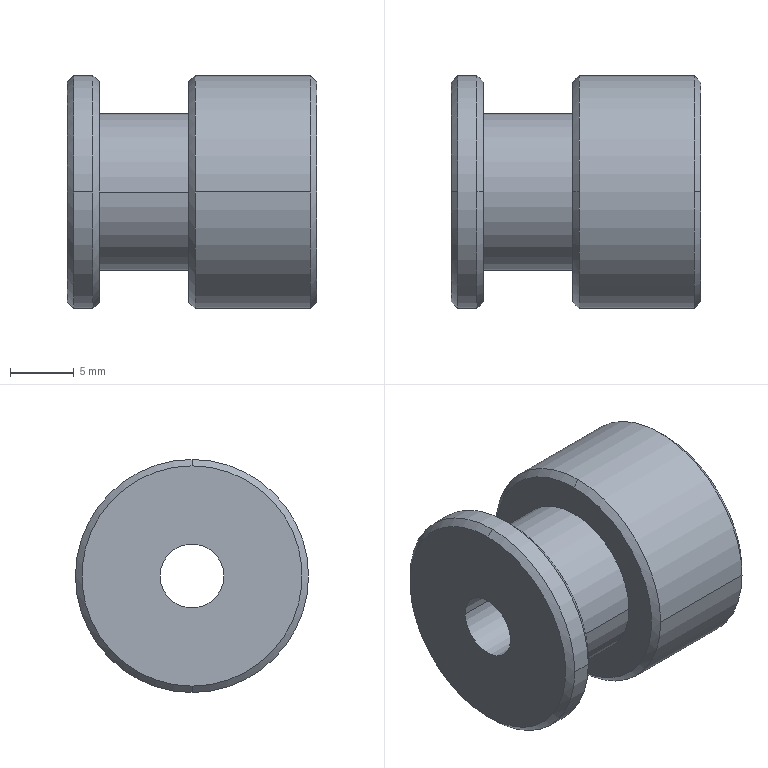Part | SolidWorks | features BaseBody 1 | 1 solid | 20 faces | box 19.5 x 18.22 x 18.22 mm | volume 3669 mm3 | cylinder 8 | cone 8 | plane 4 | commonest cylinder face diameters 18.22 x4 5 x2 12.22 x2
STEP:
#1=CARTESIAN_POINT('',(-10.344,-4.715,9.11));
#2=VERTEX_POINT('',#1);
#3=CARTESIAN_POINT('',(-10.344,-13.825,0.));
#4=VERTEX_POINT('',#3);
#5=CARTESIAN_POINT('',(-10.344,-4.715,0.));
#6=DIRECTION('',(1.,0.,0.));
#7=DIRECTION('',(0.,1.,0.));
#8=AXIS2_PLACEMENT_3D('',#5,#6,#7);
#9=CIRCLE('',#8,9.11);
#10=EDGE_CURVE('',#2,#4,#9,.T.);
#11=ORIENTED_EDGE('',*,*,#10,.T.);
#12=CARTESIAN_POINT('',(-1.344,-13.825,0.));
#13=VERTEX_POINT('',#12);
#14=CARTESIAN_POINT('',(-5.844,-13.825,0.));
#15=DIRECTION('',(1.,0.,0.));
#16=VECTOR('',#15,1000.);
#17=LINE('',#14,#16);
#18=EDGE_CURVE('',#4,#13,#17,.T.);
#19=ORIENTED_EDGE('',*,*,#18,.T.);
#20=CARTESIAN_POINT('',(-1.344,-4.715,9.11));
#21=VERTEX_POINT('',#20);
#22=CARTESIAN_POINT('',(-1.344,-4.715,0.));
#23=DIRECTION('',(-1.,0.,0.));
#24=DIRECTION('',(0.,1.,0.));
#25=AXIS2_PLACEMENT_3D('',#22,#23,#24);
#26=CIRCLE('',#25,9.11);
#27=EDGE_CURVE('',#13,#21,#26,.T.);
#28=ORIENTED_EDGE('',*,*,#27,.T.);
#29=CARTESIAN_POINT('',(-1.344,4.395,0.));
#30=VERTEX_POINT('',#29);
#31=CARTESIAN_POINT('',(-1.344,-4.715,0.));
#32=DIRECTION('',(-1.,0.,0.));
#33=DIRECTION('',(0.,1.,0.));
#34=AXIS2_PLACEMENT_3D('',#31,#32,#33);
#35=CIRCLE('',#34,9.11);
#36=EDGE_CURVE('',#21,#30,#35,.T.);
#37=ORIENTED_EDGE('',*,*,#36,.T.);
#38=CARTESIAN_POINT('',(-10.344,4.395,0.));
#39=VERTEX_POINT('',#38);
#40=CARTESIAN_POINT('',(-5.844,4.395,0.));
#41=DIRECTION('',(1.,0.,0.));
#42=VECTOR('',#41,1000.);
#43=LINE('',#40,#42);
#44=EDGE_CURVE('',#39,#30,#43,.T.);
#45=ORIENTED_EDGE('',*,*,#44,.F.);
#46=CARTESIAN_POINT('',(-10.344,-4.715,0.));
#47=DIRECTION('',(1.,0.,0.));
#48=DIRECTION('',(0.,1.,0.));
#49=AXIS2_PLACEMENT_3D('',#46,#47,#48);
#50=CIRCLE('',#49,9.11);
#51=EDGE_CURVE('',#39,#2,#50,.T.);
#52=ORIENTED_EDGE('',*,*,#51,.T.);
#53=EDGE_LOOP('',(#11,#19,#28,#37,#45,#52));
#54=FACE_OUTER_BOUND('',#53,.T.);
#55=CARTESIAN_POINT('',(-5.844,-4.715,0.));
#56=DIRECTION('',(1.,0.,0.));
#57=DIRECTION('',(0.,1.,0.));
#58=AXIS2_PLACEMENT_3D('',#55,#56,#57);
#59=CYLINDRICAL_SURFACE('',#58,9.11);
#60=ADVANCED_FACE('',(#54),#59,.T.);
#61=CARTESIAN_POINT('',(-0.8436,-4.715,8.61));
#62=VERTEX_POINT('',#61);
#63=CARTESIAN_POINT('',(-0.8436,-4.715,-8.61));
#64=VERTEX_POINT('',#63);
#65=CARTESIAN_POINT('',(-0.8436,-4.715,0.));
#66=DIRECTION('',(-1.,0.,0.));
#67=DIRECTION('',(0.,0.,1.));
#68=AXIS2_PLACEMENT_3D('',#65,#66,#67);
#69=CIRCLE('',#68,8.61);
#70=EDGE_CURVE('',#62,#64,#69,.T.);
#71=ORIENTED_EDGE('',*,*,#70,.T.);
#72=CARTESIAN_POINT('',(-1.344,-4.715,-9.11));
#73=VERTEX_POINT('',#72);
#74=CARTESIAN_POINT('',(-1.344,-4.715,-9.11));
#75=DIRECTION('',(-0.7071,0.,-0.7071));
#76=VECTOR('',#75,1000.);
#77=LINE('',#74,#76);
#78=EDGE_CURVE('',#64,#73,#77,.T.);
#79=ORIENTED_EDGE('',*,*,#78,.T.);
#80=CARTESIAN_POINT('',(-1.344,-4.715,0.));
#81=DIRECTION('',(-1.,0.,0.));
#82=DIRECTION('',(0.,1.,0.));
#83=AXIS2_PLACEMENT_3D('',#80,#81,#82);
#84=CIRCLE('',#83,9.11);
#85=EDGE_CURVE('',#30,#73,#84,.T.);
#86=ORIENTED_EDGE('',*,*,#85,.F.);
#87=ORIENTED_EDGE('',*,*,#36,.F.);
#88=CARTESIAN_POINT('',(-1.344,-4.715,9.11));
#89=DIRECTION('',(-0.7071,0.,0.7071));
#90=VECTOR('',#89,1000.);
#91=LINE('',#88,#90);
#92=EDGE_CURVE('',#62,#21,#91,.T.);
#93=ORIENTED_EDGE('',*,*,#92,.F.);
#94=EDGE_LOOP('',(#71,#79,#86,#87,#93));
#95=FACE_OUTER_BOUND('',#94,.T.);
#96=CARTESIAN_POINT('',(-1.344,-4.715,0.));
#97=DIRECTION('',(-1.,0.,0.));
#98=DIRECTION('',(0.,0.,1.));
#99=AXIS2_PLACEMENT_3D('',#96,#97,#98);
#100=CONICAL_SURFACE('',#99,9.11,0.7854);
#101=ADVANCED_FACE('',(#95),#100,.T.);
#102=CARTESIAN_POINT('',(-10.844,-4.715,-8.61));
#103=VERTEX_POINT('',#102);
#104=CARTESIAN_POINT('',(-10.844,-4.715,8.61));
#105=VERTEX_POINT('',#104);
#106=CARTESIAN_POINT('',(-10.844,-4.715,0.));
#107=DIRECTION('',(1.,0.,0.));
#108=DIRECTION('',(0.,0.,-1.));
#109=AXIS2_PLACEMENT_3D('',#106,#107,#108);
#110=CIRCLE('',#109,8.61);
#111=EDGE_CURVE('',#103,#105,#110,.T.);
#112=ORIENTED_EDGE('',*,*,#111,.T.);
#113=CARTESIAN_POINT('',(-10.344,-4.715,9.11));
#114=DIRECTION('',(0.7071,0.,0.7071));
#115=VECTOR('',#114,1000.);
#116=LINE('',#113,#115);
#117=EDGE_CURVE('',#105,#2,#116,.T.);
#118=ORIENTED_EDGE('',*,*,#117,.T.);
#119=ORIENTED_EDGE('',*,*,#51,.F.);
#120=CARTESIAN_POINT('',(-10.344,-4.715,-9.11));
#121=VERTEX_POINT('',#120);
#122=CARTESIAN_POINT('',(-10.344,-4.715,0.));
#123=DIRECTION('',(1.,0.,0.));
#124=DIRECTION('',(0.,1.,0.));
#125=AXIS2_PLACEMENT_3D('',#122,#123,#124);
#126=CIRCLE('',#125,9.11);
#127=EDGE_CURVE('',#121,#39,#126,.T.);
#128=ORIENTED_EDGE('',*,*,#127,.F.);
#129=CARTESIAN_POINT('',(-10.344,-4.715,-9.11));
#130=DIRECTION('',(0.7071,0.,-0.7071));
#131=VECTOR('',#130,1000.);
#132=LINE('',#129,#131);
#133=EDGE_CURVE('',#103,#121,#132,.T.);
#134=ORIENTED_EDGE('',*,*,#133,.F.);
#135=EDGE_LOOP('',(#112,#118,#119,#128,#134));
#136=FACE_OUTER_BOUND('',#135,.T.);
#137=CARTESIAN_POINT('',(-10.344,-4.715,0.));
#138=DIRECTION('',(1.,0.,0.));
#139=DIRECTION('',(0.,0.,-1.));
#140=AXIS2_PLACEMENT_3D('',#137,#138,#139);
#141=CONICAL_SURFACE('',#140,9.11,0.7854);
#142=ADVANCED_FACE('',(#136),#141,.T.);
#143=CARTESIAN_POINT('',(-20.344,-7.215,0.));
#144=VERTEX_POINT('',#143);
#145=CARTESIAN_POINT('',(-20.344,-2.215,0.));
#146=VERTEX_POINT('',#145);
#147=CARTESIAN_POINT('',(-20.344,-4.715,0.));
#148=DIRECTION('',(1.,0.,0.));
#149=DIRECTION('',(0.,1.,0.));
#150=AXIS2_PLACEMENT_3D('',#147,#148,#149);
#151=CIRCLE('',#150,2.5);
#152=EDGE_CURVE('',#144,#146,#151,.T.);
#153=ORIENTED_EDGE('',*,*,#152,.F.);
#154=CARTESIAN_POINT('',(-0.8436,-7.215,0.));
#155=VERTEX_POINT('',#154);
#156=CARTESIAN_POINT('',(-10.594,-7.215,0.));
#157=DIRECTION('',(1.,0.,0.));
#158=VECTOR('',#157,1000.);
#159=LINE('',#156,#158);
#160=EDGE_CURVE('',#144,#155,#159,.T.);
#161=ORIENTED_EDGE('',*,*,#160,.T.);
#162=CARTESIAN_POINT('',(-0.8436,-2.215,0.));
#163=VERTEX_POINT('',#162);
#164=CARTESIAN_POINT('',(-0.8436,-4.715,0.));
#165=DIRECTION('',(-1.,0.,0.));
#166=DIRECTION('',(0.,1.,0.));
#167=AXIS2_PLACEMENT_3D('',#164,#165,#166);
#168=CIRCLE('',#167,2.5);
#169=EDGE_CURVE('',#163,#155,#168,.T.);
#170=ORIENTED_EDGE('',*,*,#169,.F.);
#171=CARTESIAN_POINT('',(-10.594,-2.215,0.));
#172=DIRECTION('',(1.,0.,0.));
#173=VECTOR('',#172,1000.);
#174=LINE('',#171,#173);
#175=EDGE_CURVE('',#146,#163,#174,.T.);
#176=ORIENTED_EDGE('',*,*,#175,.F.);
#177=EDGE_LOOP('',(#153,#161,#170,#176));
#178=FACE_OUTER_BOUND('',#177,.T.);
#179=CARTESIAN_POINT('',(-10.594,-4.715,0.));
#180=DIRECTION('',(1.,0.,0.));
#181=DIRECTION('',(0.,1.,0.));
#182=AXIS2_PLACEMENT_3D('',#179,#180,#181);
#183=CYLINDRICAL_SURFACE('',#182,2.5);
#184=ADVANCED_FACE('',(#178),#183,.F.);
#185=CARTESIAN_POINT('',(-17.844,1.395,0.));
#186=VERTEX_POINT('',#185);
#187=CARTESIAN_POINT('',(-17.844,-10.825,0.));
#188=VERTEX_POINT('',#187);
#189=CARTESIAN_POINT('',(-17.844,-4.715,0.));
#190=DIRECTION('',(1.,0.,0.));
#191=DIRECTION('',(0.,1.,0.));
#192=AXIS2_PLACEMENT_3D('',#189,#190,#191);
#193=CIRCLE('',#192,6.11);
#194=EDGE_CURVE('',#186,#188,#193,.T.);
#195=ORIENTED_EDGE('',*,*,#194,.T.);
#196=CARTESIAN_POINT('',(-10.844,-10.825,0.));
#197=VERTEX_POINT('',#196);
#198=CARTESIAN_POINT('',(-14.344,-10.825,0.));
#199=DIRECTION('',(1.,0.,0.));
#200=VECTOR('',#199,1000.);
#201=LINE('',#198,#200);
#202=EDGE_CURVE('',#188,#197,#201,.T.);
#203=ORIENTED_EDGE('',*,*,#202,.T.);
#204=CARTESIAN_POINT('',(-10.844,1.395,0.));
#205=VERTEX_POINT('',#204);
#206=CARTESIAN_POINT('',(-10.844,-4.715,0.));
#207=DIRECTION('',(1.,0.,0.));
#208=DIRECTION('',(0.,1.,0.));
#209=AXIS2_PLACEMENT_3D('',#206,#207,#208);
#210=CIRCLE('',#209,6.11);
#211=EDGE_CURVE('',#205,#197,#210,.T.);
#212=ORIENTED_EDGE('',*,*,#211,.F.);
#213=CARTESIAN_POINT('',(-14.344,1.395,0.));
#214=DIRECTION('',(1.,0.,0.));
#215=VECTOR('',#214,1000.);
#216=LINE('',#213,#215);
#217=EDGE_CURVE('',#186,#205,#216,.T.);
#218=ORIENTED_EDGE('',*,*,#217,.F.);
#219=EDGE_LOOP('',(#195,#203,#212,#218));
#220=FACE_OUTER_BOUND('',#219,.T.);
#221=CARTESIAN_POINT('',(-14.344,-4.715,0.));
#222=DIRECTION('',(1.,0.,0.));
#223=DIRECTION('',(0.,1.,0.));
#224=AXIS2_PLACEMENT_3D('',#221,#222,#223);
#225=CYLINDRICAL_SURFACE('',#224,6.11);
#226=ADVANCED_FACE('',(#220),#225,.T.);
#227=CARTESIAN_POINT('',(-20.344,-4.715,8.61));
#228=VERTEX_POINT('',#227);
#229=CARTESIAN_POINT('',(-20.344,-4.715,-8.61));
#230=VERTEX_POINT('',#229);
#231=CARTESIAN_POINT('',(-20.344,-4.715,0.));
#232=DIRECTION('',(-1.,0.,0.));
#233=DIRECTION('',(0.,0.,-1.));
#234=AXIS2_PLACEMENT_3D('',#231,#232,#233);
#235=CIRCLE('',#234,8.61);
#236=EDGE_CURVE('',#228,#230,#235,.T.);
#237=ORIENTED_EDGE('',*,*,#236,.F.);
#238=CARTESIAN_POINT('',(-19.844,-4.715,9.11));
#239=VERTEX_POINT('',#238);
#240=CARTESIAN_POINT('',(-19.844,-4.715,9.11));
#241=DIRECTION('',(0.7071,0.,0.7071));
#242=VECTOR('',#241,1000.);
#243=LINE('',#240,#242);
#244=EDGE_CURVE('',#228,#239,#243,.T.);
#245=ORIENTED_EDGE('',*,*,#244,.T.);
#246=CARTESIAN_POINT('',(-19.844,4.395,0.));
#247=VERTEX_POINT('',#246);
#248=CARTESIAN_POINT('',(-19.844,-4.715,0.));
#249=DIRECTION('',(-1.,0.,0.));
#250=DIRECTION('',(0.,-1.,0.));
#251=AXIS2_PLACEMENT_3D('',#248,#249,#250);
#252=CIRCLE('',#251,9.11);
#253=EDGE_CURVE('',#239,#247,#252,.T.);
#254=ORIENTED_EDGE('',*,*,#253,.T.);
#255=CARTESIAN_POINT('',(-19.844,-4.715,-9.11));
#256=VERTEX_POINT('',#255);
#257=CARTESIAN_POINT('',(-19.844,-4.715,0.));
#258=DIRECTION('',(-1.,0.,0.));
#259=DIRECTION('',(0.,-1.,0.));
#260=AXIS2_PLACEMENT_3D('',#257,#258,#259);
#261=CIRCLE('',#260,9.11);
#262=EDGE_CURVE('',#247,#256,#261,.T.);
#263=ORIENTED_EDGE('',*,*,#262,.T.);
#264=CARTESIAN_POINT('',(-19.844,-4.715,-9.11));
#265=DIRECTION('',(0.7071,0.,-0.7071));
#266=VECTOR('',#265,1000.);
#267=LINE('',#264,#266);
#268=EDGE_CURVE('',#230,#256,#267,.T.);
#269=ORIENTED_EDGE('',*,*,#268,.F.);
#270=EDGE_LOOP('',(#237,#245,#254,#263,#269));
#271=FACE_OUTER_BOUND('',#270,.T.);
#272=CARTESIAN_POINT('',(-19.844,-4.715,0.));
#273=DIRECTION('',(1.,0.,0.));
#274=DIRECTION('',(0.,0.,-1.));
#275=AXIS2_PLACEMENT_3D('',#272,#273,#274);
#276=CONICAL_SURFACE('',#275,9.11,0.7854);
#277=ADVANCED_FACE('',(#271),#276,.T.);
#278=CARTESIAN_POINT('',(-17.844,-4.715,-8.61));
#279=VERTEX_POINT('',#278);
#280=CARTESIAN_POINT('',(-17.844,-4.715,8.61));
#281=VERTEX_POINT('',#280);
#282=CARTESIAN_POINT('',(-17.844,-4.715,0.));
#283=DIRECTION('',(1.,0.,0.));
#284=DIRECTION('',(0.,0.,1.));
#285=AXIS2_PLACEMENT_3D('',#282,#283,#284);
#286=CIRCLE('',#285,8.61);
#287=EDGE_CURVE('',#279,#281,#286,.T.);
#288=ORIENTED_EDGE('',*,*,#287,.F.);
#289=CARTESIAN_POINT('',(-18.344,-4.715,-9.11));
#290=VERTEX_POINT('',#289);
#291=CARTESIAN_POINT('',(-18.344,-4.715,-9.11));
#292=DIRECTION('',(-0.7071,0.,-0.7071));
#293=VECTOR('',#292,1000.);
#294=LINE('',#291,#293);
#295=EDGE_CURVE('',#279,#290,#294,.T.);
#296=ORIENTED_EDGE('',*,*,#295,.T.);
#297=CARTESIAN_POINT('',(-18.344,4.395,0.));
#298=VERTEX_POINT('',#297);
#299=CARTESIAN_POINT('',(-18.344,-4.715,0.));
#300=DIRECTION('',(1.,0.,0.));
#301=DIRECTION('',(0.,-1.,0.));
#302=AXIS2_PLACEMENT_3D('',#299,#300,#301);
#303=CIRCLE('',#302,9.11);
#304=EDGE_CURVE('',#290,#298,#303,.T.);
#305=ORIENTED_EDGE('',*,*,#304,.T.);
#306=CARTESIAN_POINT('',(-18.344,-4.715,9.11));
#307=VERTEX_POINT('',#306);
#308=CARTESIAN_POINT('',(-18.344,-4.715,0.));
#309=DIRECTION('',(1.,0.,0.));
#310=DIRECTION('',(0.,-1.,0.));
#311=AXIS2_PLACEMENT_3D('',#308,#309,#310);
#312=CIRCLE('',#311,9.11);
#313=EDGE_CURVE('',#298,#307,#312,.T.);
#314=ORIENTED_EDGE('',*,*,#313,.T.);
#315=CARTESIAN_POINT('',(-18.344,-4.715,9.11));
#316=DIRECTION('',(-0.7071,0.,0.7071));
#317=VECTOR('',#316,1000.);
#318=LINE('',#315,#317);
#319=EDGE_CURVE('',#281,#307,#318,.T.);
#320=ORIENTED_EDGE('',*,*,#319,.F.);
#321=EDGE_LOOP('',(#288,#296,#305,#314,#320));
#322=FACE_OUTER_BOUND('',#321,.T.);
#323=CARTESIAN_POINT('',(-18.344,-4.715,0.));
#324=DIRECTION('',(-1.,0.,0.));
#325=DIRECTION('',(0.,0.,1.));
#326=AXIS2_PLACEMENT_3D('',#323,#324,#325);
#327=CONICAL_SURFACE('',#326,9.11,0.7854);
#328=ADVANCED_FACE('',(#322),#327,.T.);
#329=CARTESIAN_POINT('',(-19.844,-13.825,0.));
#330=VERTEX_POINT('',#329);
#331=CARTESIAN_POINT('',(-19.844,-4.715,0.));
#332=DIRECTION('',(-1.,0.,0.));
#333=DIRECTION('',(0.,-1.,0.));
#334=AXIS2_PLACEMENT_3D('',#331,#332,#333);
#335=CIRCLE('',#334,9.11);
#336=EDGE_CURVE('',#330,#239,#335,.T.);
#337=ORIENTED_EDGE('',*,*,#336,.F.);
#338=CARTESIAN_POINT('',(-18.344,-13.825,0.));
#339=VERTEX_POINT('',#338);
#340=CARTESIAN_POINT('',(-19.094,-13.825,0.));
#341=DIRECTION('',(1.,0.,0.));
#342=VECTOR('',#341,1000.);
#343=LINE('',#340,#342);
#344=EDGE_CURVE('',#330,#339,#343,.T.);
#345=ORIENTED_EDGE('',*,*,#344,.T.);
#346=CARTESIAN_POINT('',(-18.344,-4.715,0.));
#347=DIRECTION('',(1.,0.,0.));
#348=DIRECTION('',(0.,-1.,0.));
#349=AXIS2_PLACEMENT_3D('',#346,#347,#348);
#350=CIRCLE('',#349,9.11);
#351=EDGE_CURVE('',#307,#339,#350,.T.);
#352=ORIENTED_EDGE('',*,*,#351,.F.);
#353=ORIENTED_EDGE('',*,*,#313,.F.);
#354=CARTESIAN_POINT('',(-19.094,4.395,0.));
#355=DIRECTION('',(1.,0.,0.));
#356=VECTOR('',#355,1000.);
#357=LINE('',#354,#356);
#358=EDGE_CURVE('',#247,#298,#357,.T.);
#359=ORIENTED_EDGE('',*,*,#358,.F.);
#360=ORIENTED_EDGE('',*,*,#253,.F.);
#361=EDGE_LOOP('',(#337,#345,#352,#353,#359,#360));
#362=FACE_OUTER_BOUND('',#361,.T.);
#363=CARTESIAN_POINT('',(-19.094,-4.715,0.));
#364=DIRECTION('',(1.,0.,0.));
#365=DIRECTION('',(0.,1.,0.));
#366=AXIS2_PLACEMENT_3D('',#363,#364,#365);
#367=CYLINDRICAL_SURFACE('',#366,9.11);
#368=ADVANCED_FACE('',(#362),#367,.T.);
#369=ORIENTED_EDGE('',*,*,#18,.F.);
#370=CARTESIAN_POINT('',(-10.344,-4.715,0.));
#371=DIRECTION('',(1.,0.,0.));
#372=DIRECTION('',(0.,1.,0.));
#373=AXIS2_PLACEMENT_3D('',#370,#371,#372);
#374=CIRCLE('',#373,9.11);
#375=EDGE_CURVE('',#4,#121,#374,.T.);
#376=ORIENTED_EDGE('',*,*,#375,.T.);
#377=ORIENTED_EDGE('',*,*,#127,.T.);
#378=ORIENTED_EDGE('',*,*,#44,.T.);
#379=ORIENTED_EDGE('',*,*,#85,.T.);
#380=CARTESIAN_POINT('',(-1.344,-4.715,0.));
#381=DIRECTION('',(-1.,0.,0.));
#382=DIRECTION('',(0.,1.,0.));
#383=AXIS2_PLACEMENT_3D('',#380,#381,#382);
#384=CIRCLE('',#383,9.11);
#385=EDGE_CURVE('',#73,#13,#384,.T.);
#386=ORIENTED_EDGE('',*,*,#385,.T.);
#387=EDGE_LOOP('',(#369,#376,#377,#378,#379,#386));
#388=FACE_OUTER_BOUND('',#387,.T.);
#389=CARTESIAN_POINT('',(-5.844,-4.715,0.));
#390=DIRECTION('',(1.,0.,0.));
#391=DIRECTION('',(0.,1.,0.));
#392=AXIS2_PLACEMENT_3D('',#389,#390,#391);
#393=CYLINDRICAL_SURFACE('',#392,9.11);
#394=ADVANCED_FACE('',(#388),#393,.T.);
#395=ORIENTED_EDGE('',*,*,#78,.F.);
#396=CARTESIAN_POINT('',(-0.8436,-4.715,0.));
#397=DIRECTION('',(-1.,0.,0.));
#398=DIRECTION('',(0.,0.,1.));
#399=AXIS2_PLACEMENT_3D('',#396,#397,#398);
#400=CIRCLE('',#399,8.61);
#401=EDGE_CURVE('',#64,#62,#400,.T.);
#402=ORIENTED_EDGE('',*,*,#401,.T.);
#403=ORIENTED_EDGE('',*,*,#92,.T.);
#404=ORIENTED_EDGE('',*,*,#27,.F.);
#405=ORIENTED_EDGE('',*,*,#385,.F.);
#406=EDGE_LOOP('',(#395,#402,#403,#404,#405));
#407=FACE_OUTER_BOUND('',#406,.T.);
#408=CARTESIAN_POINT('',(-1.344,-4.715,0.));
#409=DIRECTION('',(-1.,0.,0.));
#410=DIRECTION('',(0.,0.,1.));
#411=AXIS2_PLACEMENT_3D('',#408,#409,#410);
#412=CONICAL_SURFACE('',#411,9.11,0.7854);
#413=ADVANCED_FACE('',(#407),#412,.T.);
#414=ORIENTED_EDGE('',*,*,#117,.F.);
#415=CARTESIAN_POINT('',(-10.844,-4.715,0.));
#416=DIRECTION('',(1.,0.,0.));
#417=DIRECTION('',(0.,0.,-1.));
#418=AXIS2_PLACEMENT_3D('',#415,#416,#417);
#419=CIRCLE('',#418,8.61);
#420=EDGE_CURVE('',#105,#103,#419,.T.);
#421=ORIENTED_EDGE('',*,*,#420,.T.);
#422=ORIENTED_EDGE('',*,*,#133,.T.);
#423=ORIENTED_EDGE('',*,*,#375,.F.);
#424=ORIENTED_EDGE('',*,*,#10,.F.);
#425=EDGE_LOOP('',(#414,#421,#422,#423,#424));
#426=FACE_OUTER_BOUND('',#425,.T.);
#427=CARTESIAN_POINT('',(-10.344,-4.715,0.));
#428=DIRECTION('',(1.,0.,0.));
#429=DIRECTION('',(0.,0.,-1.));
#430=AXIS2_PLACEMENT_3D('',#427,#428,#429);
#431=CONICAL_SURFACE('',#430,9.11,0.7854);
#432=ADVANCED_FACE('',(#426),#431,.T.);
#433=ORIENTED_EDGE('',*,*,#169,.T.);
#434=CARTESIAN_POINT('',(-0.8436,-4.715,0.));
#435=DIRECTION('',(-1.,0.,0.));
#436=DIRECTION('',(0.,1.,0.));
#437=AXIS2_PLACEMENT_3D('',#434,#435,#436);
#438=CIRCLE('',#437,2.5);
#439=EDGE_CURVE('',#155,#163,#438,.T.);
#440=ORIENTED_EDGE('',*,*,#439,.T.);
#441=EDGE_LOOP('',(#433,#440));
#442=FACE_BOUND('',#441,.T.);
#443=ORIENTED_EDGE('',*,*,#70,.F.);
#444=ORIENTED_EDGE('',*,*,#401,.F.);
#445=EDGE_LOOP('',(#443,#444));
#446=FACE_OUTER_BOUND('',#445,.T.);
#447=CARTESIAN_POINT('',(-0.8436,1.09,0.));
#448=DIRECTION('',(1.,0.,0.));
#449=DIRECTION('',(0.,0.,-1.));
#450=AXIS2_PLACEMENT_3D('',#447,#448,#449);
#451=PLANE('',#450);
#452=ADVANCED_FACE('',(#442,#446),#451,.T.);
#453=ORIENTED_EDGE('',*,*,#211,.T.);
#454=CARTESIAN_POINT('',(-10.844,-4.715,0.));
#455=DIRECTION('',(1.,0.,0.));
#456=DIRECTION('',(0.,1.,0.));
#457=AXIS2_PLACEMENT_3D('',#454,#455,#456);
#458=CIRCLE('',#457,6.11);
#459=EDGE_CURVE('',#197,#205,#458,.T.);
#460=ORIENTED_EDGE('',*,*,#459,.T.);
#461=EDGE_LOOP('',(#453,#460));
#462=FACE_BOUND('',#461,.T.);
#463=ORIENTED_EDGE('',*,*,#111,.F.);
#464=ORIENTED_EDGE('',*,*,#420,.F.);
#465=EDGE_LOOP('',(#463,#464));
#466=FACE_OUTER_BOUND('',#465,.T.);
#467=CARTESIAN_POINT('',(-10.844,2.895,0.));
#468=DIRECTION('',(-1.,0.,0.));
#469=DIRECTION('',(0.,0.,1.));
#470=AXIS2_PLACEMENT_3D('',#467,#468,#469);
#471=PLANE('',#470);
#472=ADVANCED_FACE('',(#462,#466),#471,.T.);
#473=ORIENTED_EDGE('',*,*,#160,.F.);
#474=CARTESIAN_POINT('',(-20.344,-4.715,0.));
#475=DIRECTION('',(1.,0.,0.));
#476=DIRECTION('',(0.,1.,0.));
#477=AXIS2_PLACEMENT_3D('',#474,#475,#476);
#478=CIRCLE('',#477,2.5);
#479=EDGE_CURVE('',#146,#144,#478,.T.);
#480=ORIENTED_EDGE('',*,*,#479,.F.);
#481=ORIENTED_EDGE('',*,*,#175,.T.);
#482=ORIENTED_EDGE('',*,*,#439,.F.);
#483=EDGE_LOOP('',(#473,#480,#481,#482));
#484=FACE_OUTER_BOUND('',#483,.T.);
#485=CARTESIAN_POINT('',(-10.594,-4.715,0.));
#486=DIRECTION('',(1.,0.,0.));
#487=DIRECTION('',(0.,1.,0.));
#488=AXIS2_PLACEMENT_3D('',#485,#486,#487);
#489=CYLINDRICAL_SURFACE('',#488,2.5);
#490=ADVANCED_FACE('',(#484),#489,.F.);
#491=ORIENTED_EDGE('',*,*,#202,.F.);
#492=CARTESIAN_POINT('',(-17.844,-4.715,0.));
#493=DIRECTION('',(1.,0.,0.));
#494=DIRECTION('',(0.,1.,0.));
#495=AXIS2_PLACEMENT_3D('',#492,#493,#494);
#496=CIRCLE('',#495,6.11);
#497=EDGE_CURVE('',#188,#186,#496,.T.);
#498=ORIENTED_EDGE('',*,*,#497,.T.);
#499=ORIENTED_EDGE('',*,*,#217,.T.);
#500=ORIENTED_EDGE('',*,*,#459,.F.);
#501=EDGE_LOOP('',(#491,#498,#499,#500));
#502=FACE_OUTER_BOUND('',#501,.T.);
#503=CARTESIAN_POINT('',(-14.344,-4.715,0.));
#504=DIRECTION('',(1.,0.,0.));
#505=DIRECTION('',(0.,1.,0.));
#506=AXIS2_PLACEMENT_3D('',#503,#504,#505);
#507=CYLINDRICAL_SURFACE('',#506,6.11);
#508=ADVANCED_FACE('',(#502),#507,.T.);
#509=ORIENTED_EDGE('',*,*,#479,.T.);
#510=ORIENTED_EDGE('',*,*,#152,.T.);
#511=EDGE_LOOP('',(#509,#510));
#512=FACE_BOUND('',#511,.T.);
#513=CARTESIAN_POINT('',(-20.344,-4.715,0.));
#514=DIRECTION('',(-1.,0.,0.));
#515=DIRECTION('',(0.,0.,-1.));
#516=AXIS2_PLACEMENT_3D('',#513,#514,#515);
#517=CIRCLE('',#516,8.61);
#518=EDGE_CURVE('',#230,#228,#517,.T.);
#519=ORIENTED_EDGE('',*,*,#518,.T.);
#520=ORIENTED_EDGE('',*,*,#236,.T.);
#521=EDGE_LOOP('',(#519,#520));
#522=FACE_OUTER_BOUND('',#521,.T.);
#523=CARTESIAN_POINT('',(-20.344,1.09,0.));
#524=DIRECTION('',(-1.,0.,0.));
#525=DIRECTION('',(0.,0.,1.));
#526=AXIS2_PLACEMENT_3D('',#523,#524,#525);
#527=PLANE('',#526);
#528=ADVANCED_FACE('',(#512,#522),#527,.T.);
#529=ORIENTED_EDGE('',*,*,#194,.F.);
#530=ORIENTED_EDGE('',*,*,#497,.F.);
#531=EDGE_LOOP('',(#529,#530));
#532=FACE_BOUND('',#531,.T.);
#533=CARTESIAN_POINT('',(-17.844,-4.715,0.));
#534=DIRECTION('',(1.,0.,0.));
#535=DIRECTION('',(0.,0.,1.));
#536=AXIS2_PLACEMENT_3D('',#533,#534,#535);
#537=CIRCLE('',#536,8.61);
#538=EDGE_CURVE('',#281,#279,#537,.T.);
#539=ORIENTED_EDGE('',*,*,#538,.T.);
#540=ORIENTED_EDGE('',*,*,#287,.T.);
#541=EDGE_LOOP('',(#539,#540));
#542=FACE_OUTER_BOUND('',#541,.T.);
#543=CARTESIAN_POINT('',(-17.844,2.895,0.));
#544=DIRECTION('',(1.,0.,0.));
#545=DIRECTION('',(0.,0.,-1.));
#546=AXIS2_PLACEMENT_3D('',#543,#544,#545);
#547=PLANE('',#546);
#548=ADVANCED_FACE('',(#532,#542),#547,.T.);
#549=ORIENTED_EDGE('',*,*,#244,.F.);
#550=ORIENTED_EDGE('',*,*,#518,.F.);
#551=ORIENTED_EDGE('',*,*,#268,.T.);
#552=CARTESIAN_POINT('',(-19.844,-4.715,0.));
#553=DIRECTION('',(-1.,0.,0.));
#554=DIRECTION('',(0.,-1.,0.));
#555=AXIS2_PLACEMENT_3D('',#552,#553,#554);
#556=CIRCLE('',#555,9.11);
#557=EDGE_CURVE('',#256,#330,#556,.T.);
#558=ORIENTED_EDGE('',*,*,#557,.T.);
#559=ORIENTED_EDGE('',*,*,#336,.T.);
#560=EDGE_LOOP('',(#549,#550,#551,#558,#559));
#561=FACE_OUTER_BOUND('',#560,.T.);
#562=CARTESIAN_POINT('',(-19.844,-4.715,0.));
#563=DIRECTION('',(1.,0.,0.));
#564=DIRECTION('',(0.,0.,-1.));
#565=AXIS2_PLACEMENT_3D('',#562,#563,#564);
#566=CONICAL_SURFACE('',#565,9.11,0.7854);
#567=ADVANCED_FACE('',(#561),#566,.T.);
#568=ORIENTED_EDGE('',*,*,#295,.F.);
#569=ORIENTED_EDGE('',*,*,#538,.F.);
#570=ORIENTED_EDGE('',*,*,#319,.T.);
#571=ORIENTED_EDGE('',*,*,#351,.T.);
#572=CARTESIAN_POINT('',(-18.344,-4.715,0.));
#573=DIRECTION('',(1.,0.,0.));
#574=DIRECTION('',(0.,-1.,0.));
#575=AXIS2_PLACEMENT_3D('',#572,#573,#574);
#576=CIRCLE('',#575,9.11);
#577=EDGE_CURVE('',#339,#290,#576,.T.);
#578=ORIENTED_EDGE('',*,*,#577,.T.);
#579=EDGE_LOOP('',(#568,#569,#570,#571,#578));
#580=FACE_OUTER_BOUND('',#579,.T.);
#581=CARTESIAN_POINT('',(-18.344,-4.715,0.));
#582=DIRECTION('',(-1.,0.,0.));
#583=DIRECTION('',(0.,0.,1.));
#584=AXIS2_PLACEMENT_3D('',#581,#582,#583);
#585=CONICAL_SURFACE('',#584,9.11,0.7854);
#586=ADVANCED_FACE('',(#580),#585,.T.);
#587=ORIENTED_EDGE('',*,*,#344,.F.);
#588=ORIENTED_EDGE('',*,*,#557,.F.);
#589=ORIENTED_EDGE('',*,*,#262,.F.);
#590=ORIENTED_EDGE('',*,*,#358,.T.);
#591=ORIENTED_EDGE('',*,*,#304,.F.);
#592=ORIENTED_EDGE('',*,*,#577,.F.);
#593=EDGE_LOOP('',(#587,#588,#589,#590,#591,#592));
#594=FACE_OUTER_BOUND('',#593,.T.);
#595=CARTESIAN_POINT('',(-19.094,-4.715,0.));
#596=DIRECTION('',(1.,0.,0.));
#597=DIRECTION('',(0.,1.,0.));
#598=AXIS2_PLACEMENT_3D('',#595,#596,#597);
#599=CYLINDRICAL_SURFACE('',#598,9.11);
#600=ADVANCED_FACE('',(#594),#599,.T.);
#601=CLOSED_SHELL('',(#60,#101,#142,#184,#226,#277,#328,#368,#394,#413,#432,#452,#472,#490,#508,#528,#548,#567,#586,#600));
#602=MANIFOLD_SOLID_BREP('',#601);
#603=CARTESIAN_POINT('',(0.,0.,0.));
#604=DIRECTION('',(0.,0.,1.));
#605=DIRECTION('',(1.,0.,0.));
#606=AXIS2_PLACEMENT_3D('',#603,#604,#605);
#607=(LENGTH_UNIT()NAMED_UNIT(*)SI_UNIT(.MILLI.,.METRE.));
#608=UNCERTAINTY_MEASURE_WITH_UNIT(LENGTH_MEASURE(0.00001),#607,'','');
#609=(NAMED_UNIT(*)PLANE_ANGLE_UNIT()SI_UNIT($,.RADIAN.));
#610=(NAMED_UNIT(*)SI_UNIT($,.STERADIAN.)SOLID_ANGLE_UNIT());
#611=(GEOMETRIC_REPRESENTATION_CONTEXT(3)GLOBAL_UNCERTAINTY_ASSIGNED_CONTEXT((#608))GLOBAL_UNIT_ASSIGNED_CONTEXT((#607,#609,#610))REPRESENTATION_CONTEXT('',''));
#612=ADVANCED_BREP_SHAPE_REPRESENTATION('',(#602,#606),#611);